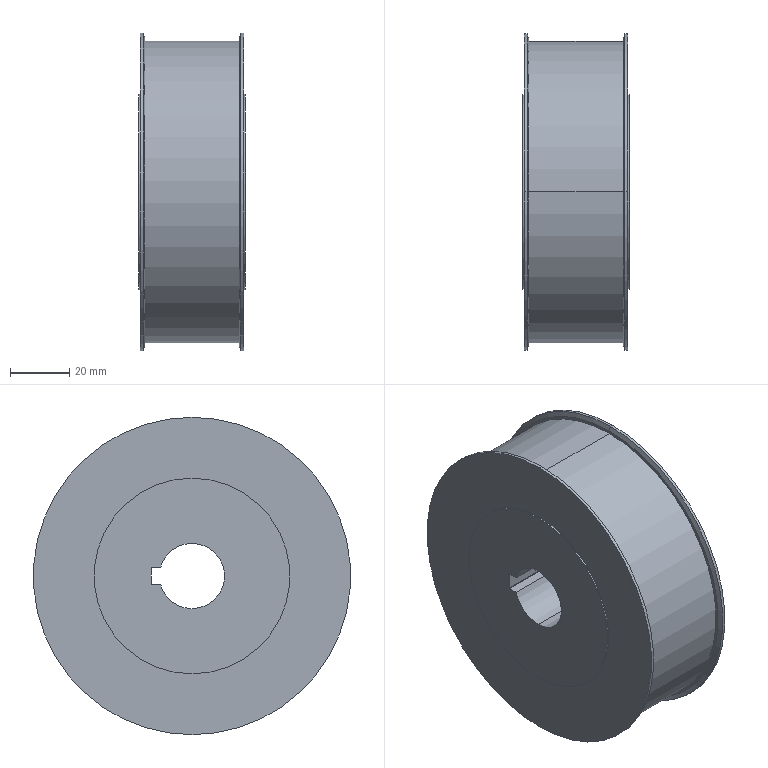Part | SolidWorks | features ICE 3, Fillet 1, Revolution 1 | 1 solid | 35 faces | box 36 x 107 x 107 mm | volume 274839 mm3 | cylinder 20 | plane 11 | cone 4 | commonest cylinder face diameters 66 x4 107 x4 22 x3 24.5 x3 0.4 x2 35 x2
STEP:
#1=CARTESIAN_POINT('',(11.,0.,12.25));
#2=VERTEX_POINT('',#1);
#3=CARTESIAN_POINT('',(11.,0.,-12.25));
#4=VERTEX_POINT('',#3);
#5=CARTESIAN_POINT('',(11.,0.,0.));
#6=DIRECTION('',(1.,0.,0.));
#7=DIRECTION('',(0.,0.,-1.));
#8=AXIS2_PLACEMENT_3D('',#5,#6,#7);
#9=CIRCLE('',#8,12.25);
#10=EDGE_CURVE('',#2,#4,#9,.T.);
#11=ORIENTED_EDGE('',*,*,#10,.F.);
#12=CARTESIAN_POINT('',(16.,0.,12.25));
#13=VERTEX_POINT('',#12);
#14=CARTESIAN_POINT('',(11.,0.,12.25));
#15=DIRECTION('',(1.,0.,0.));
#16=VECTOR('',#15,1000.);
#17=LINE('',#14,#16);
#18=EDGE_CURVE('',#2,#13,#17,.T.);
#19=ORIENTED_EDGE('',*,*,#18,.T.);
#20=CARTESIAN_POINT('',(16.,0.,-12.25));
#21=VERTEX_POINT('',#20);
#22=CARTESIAN_POINT('',(16.,0.,0.));
#23=DIRECTION('',(1.,0.,0.));
#24=DIRECTION('',(0.,0.,-1.));
#25=AXIS2_PLACEMENT_3D('',#22,#23,#24);
#26=CIRCLE('',#25,12.25);
#27=EDGE_CURVE('',#13,#21,#26,.T.);
#28=ORIENTED_EDGE('',*,*,#27,.T.);
#29=CARTESIAN_POINT('',(11.,0.,-12.25));
#30=DIRECTION('',(1.,0.,0.));
#31=VECTOR('',#30,1000.);
#32=LINE('',#29,#31);
#33=EDGE_CURVE('',#4,#21,#32,.T.);
#34=ORIENTED_EDGE('',*,*,#33,.F.);
#35=EDGE_LOOP('',(#11,#19,#28,#34));
#36=FACE_OUTER_BOUND('',#35,.T.);
#37=CARTESIAN_POINT('',(11.,0.,0.));
#38=DIRECTION('',(1.,0.,0.));
#39=DIRECTION('',(0.,0.,-1.));
#40=AXIS2_PLACEMENT_3D('',#37,#38,#39);
#41=CYLINDRICAL_SURFACE('',#40,12.25);
#42=ADVANCED_FACE('',(#36),#41,.F.);
#43=CARTESIAN_POINT('',(11.,11.877,-3.));
#44=VERTEX_POINT('',#43);
#45=CARTESIAN_POINT('',(11.,0.,0.));
#46=DIRECTION('',(1.,0.,0.));
#47=DIRECTION('',(0.,0.,-1.));
#48=AXIS2_PLACEMENT_3D('',#45,#46,#47);
#49=CIRCLE('',#48,12.25);
#50=EDGE_CURVE('',#4,#44,#49,.T.);
#51=ORIENTED_EDGE('',*,*,#50,.F.);
#52=ORIENTED_EDGE('',*,*,#33,.T.);
#53=CARTESIAN_POINT('',(16.,11.877,-3.));
#54=VERTEX_POINT('',#53);
#55=CARTESIAN_POINT('',(16.,0.,0.));
#56=DIRECTION('',(1.,0.,0.));
#57=DIRECTION('',(0.,0.,-1.));
#58=AXIS2_PLACEMENT_3D('',#55,#56,#57);
#59=CIRCLE('',#58,12.25);
#60=EDGE_CURVE('',#21,#54,#59,.T.);
#61=ORIENTED_EDGE('',*,*,#60,.T.);
#62=CARTESIAN_POINT('',(11.,11.877,-3.));
#63=DIRECTION('',(1.,0.,0.));
#64=VECTOR('',#63,1000.);
#65=LINE('',#62,#64);
#66=EDGE_CURVE('',#44,#54,#65,.T.);
#67=ORIENTED_EDGE('',*,*,#66,.F.);
#68=EDGE_LOOP('',(#51,#52,#61,#67));
#69=FACE_OUTER_BOUND('',#68,.T.);
#70=CARTESIAN_POINT('',(11.,0.,0.));
#71=DIRECTION('',(1.,0.,0.));
#72=DIRECTION('',(0.,0.,-1.));
#73=AXIS2_PLACEMENT_3D('',#70,#71,#72);
#74=CYLINDRICAL_SURFACE('',#73,12.25);
#75=ADVANCED_FACE('',(#69),#74,.F.);
#76=CARTESIAN_POINT('',(16.,0.,17.5));
#77=VERTEX_POINT('',#76);
#78=CARTESIAN_POINT('',(16.,0.,-17.5));
#79=VERTEX_POINT('',#78);
#80=CARTESIAN_POINT('',(16.,0.,0.));
#81=DIRECTION('',(1.,0.,0.));
#82=DIRECTION('',(0.,0.,-1.));
#83=AXIS2_PLACEMENT_3D('',#80,#81,#82);
#84=CIRCLE('',#83,17.5);
#85=EDGE_CURVE('',#77,#79,#84,.T.);
#86=ORIENTED_EDGE('',*,*,#85,.F.);
#87=CARTESIAN_POINT('',(18.,0.,17.5));
#88=VERTEX_POINT('',#87);
#89=CARTESIAN_POINT('',(16.,0.,17.5));
#90=DIRECTION('',(1.,0.,0.));
#91=VECTOR('',#90,1000.);
#92=LINE('',#89,#91);
#93=EDGE_CURVE('',#77,#88,#92,.T.);
#94=ORIENTED_EDGE('',*,*,#93,.T.);
#95=CARTESIAN_POINT('',(18.,0.,-17.5));
#96=VERTEX_POINT('',#95);
#97=CARTESIAN_POINT('',(18.,0.,0.));
#98=DIRECTION('',(1.,0.,0.));
#99=DIRECTION('',(0.,0.,-1.));
#100=AXIS2_PLACEMENT_3D('',#97,#98,#99);
#101=CIRCLE('',#100,17.5);
#102=EDGE_CURVE('',#88,#96,#101,.T.);
#103=ORIENTED_EDGE('',*,*,#102,.T.);
#104=CARTESIAN_POINT('',(16.,0.,-17.5));
#105=DIRECTION('',(1.,0.,0.));
#106=VECTOR('',#105,1000.);
#107=LINE('',#104,#106);
#108=EDGE_CURVE('',#79,#96,#107,.T.);
#109=ORIENTED_EDGE('',*,*,#108,.F.);
#110=EDGE_LOOP('',(#86,#94,#103,#109));
#111=FACE_OUTER_BOUND('',#110,.T.);
#112=CARTESIAN_POINT('',(16.,0.,0.));
#113=DIRECTION('',(1.,0.,0.));
#114=DIRECTION('',(0.,0.,-1.));
#115=AXIS2_PLACEMENT_3D('',#112,#113,#114);
#116=CYLINDRICAL_SURFACE('',#115,17.5);
#117=ADVANCED_FACE('',(#111),#116,.F.);
#118=CARTESIAN_POINT('',(-17.5,0.,33.));
#119=VERTEX_POINT('',#118);
#120=CARTESIAN_POINT('',(-17.5,0.,-33.));
#121=VERTEX_POINT('',#120);
#122=CARTESIAN_POINT('',(-17.5,0.,0.));
#123=DIRECTION('',(-1.,0.,0.));
#124=DIRECTION('',(0.,0.,1.));
#125=AXIS2_PLACEMENT_3D('',#122,#123,#124);
#126=CIRCLE('',#125,33.);
#127=EDGE_CURVE('',#119,#121,#126,.T.);
#128=ORIENTED_EDGE('',*,*,#127,.T.);
#129=CARTESIAN_POINT('',(-18.,0.,-33.));
#130=VERTEX_POINT('',#129);
#131=CARTESIAN_POINT('',(-18.,0.,-33.));
#132=DIRECTION('',(-1.,0.,0.));
#133=VECTOR('',#132,1000.);
#134=LINE('',#131,#133);
#135=EDGE_CURVE('',#121,#130,#134,.T.);
#136=ORIENTED_EDGE('',*,*,#135,.T.);
#137=CARTESIAN_POINT('',(-18.,0.,33.));
#138=VERTEX_POINT('',#137);
#139=CARTESIAN_POINT('',(-18.,0.,0.));
#140=DIRECTION('',(-1.,0.,0.));
#141=DIRECTION('',(0.,0.,1.));
#142=AXIS2_PLACEMENT_3D('',#139,#140,#141);
#143=CIRCLE('',#142,33.);
#144=EDGE_CURVE('',#138,#130,#143,.T.);
#145=ORIENTED_EDGE('',*,*,#144,.F.);
#146=CARTESIAN_POINT('',(-18.,0.,33.));
#147=DIRECTION('',(-1.,0.,0.));
#148=VECTOR('',#147,1000.);
#149=LINE('',#146,#148);
#150=EDGE_CURVE('',#119,#138,#149,.T.);
#151=ORIENTED_EDGE('',*,*,#150,.F.);
#152=EDGE_LOOP('',(#128,#136,#145,#151));
#153=FACE_OUTER_BOUND('',#152,.T.);
#154=CARTESIAN_POINT('',(-18.,0.,0.));
#155=DIRECTION('',(-1.,0.,0.));
#156=DIRECTION('',(0.,0.,1.));
#157=AXIS2_PLACEMENT_3D('',#154,#155,#156);
#158=CYLINDRICAL_SURFACE('',#157,33.);
#159=ADVANCED_FACE('',(#153),#158,.T.);
#160=CARTESIAN_POINT('',(-16.5,0.,53.5));
#161=VERTEX_POINT('',#160);
#162=CARTESIAN_POINT('',(-16.5,0.,-53.5));
#163=VERTEX_POINT('',#162);
#164=CARTESIAN_POINT('',(-16.5,0.,0.));
#165=DIRECTION('',(-1.,0.,0.));
#166=DIRECTION('',(0.,0.,1.));
#167=AXIS2_PLACEMENT_3D('',#164,#165,#166);
#168=CIRCLE('',#167,53.5);
#169=EDGE_CURVE('',#161,#163,#168,.T.);
#170=ORIENTED_EDGE('',*,*,#169,.T.);
#171=CARTESIAN_POINT('',(-17.5,0.,-53.5));
#172=VERTEX_POINT('',#171);
#173=CARTESIAN_POINT('',(-18.,0.,-53.5));
#174=DIRECTION('',(-1.,0.,0.));
#175=VECTOR('',#174,1000.);
#176=LINE('',#173,#175);
#177=EDGE_CURVE('',#163,#172,#176,.T.);
#178=ORIENTED_EDGE('',*,*,#177,.T.);
#179=CARTESIAN_POINT('',(-17.5,0.,53.5));
#180=VERTEX_POINT('',#179);
#181=CARTESIAN_POINT('',(-17.5,0.,0.));
#182=DIRECTION('',(-1.,0.,0.));
#183=DIRECTION('',(0.,0.,1.));
#184=AXIS2_PLACEMENT_3D('',#181,#182,#183);
#185=CIRCLE('',#184,53.5);
#186=EDGE_CURVE('',#180,#172,#185,.T.);
#187=ORIENTED_EDGE('',*,*,#186,.F.);
#188=CARTESIAN_POINT('',(-18.,0.,53.5));
#189=DIRECTION('',(-1.,0.,0.));
#190=VECTOR('',#189,1000.);
#191=LINE('',#188,#190);
#192=EDGE_CURVE('',#161,#180,#191,.T.);
#193=ORIENTED_EDGE('',*,*,#192,.F.);
#194=EDGE_LOOP('',(#170,#178,#187,#193));
#195=FACE_OUTER_BOUND('',#194,.T.);
#196=CARTESIAN_POINT('',(-18.,0.,0.));
#197=DIRECTION('',(-1.,0.,0.));
#198=DIRECTION('',(0.,0.,1.));
#199=AXIS2_PLACEMENT_3D('',#196,#197,#198);
#200=CYLINDRICAL_SURFACE('',#199,53.5);
#201=ADVANCED_FACE('',(#195),#200,.T.);
#202=CARTESIAN_POINT('',(-15.9,0.,51.9));
#203=VERTEX_POINT('',#202);
#204=CARTESIAN_POINT('',(-15.9,0.,-51.9));
#205=VERTEX_POINT('',#204);
#206=CARTESIAN_POINT('',(-15.9,0.,0.));
#207=DIRECTION('',(-1.,0.,0.));
#208=DIRECTION('',(0.,0.,1.));
#209=AXIS2_PLACEMENT_3D('',#206,#207,#208);
#210=CIRCLE('',#209,51.9);
#211=EDGE_CURVE('',#203,#205,#210,.T.);
#212=ORIENTED_EDGE('',*,*,#211,.T.);
#213=CARTESIAN_POINT('',(-15.9,0.,-51.9));
#214=DIRECTION('',(-0.3511,0.,-0.9363));
#215=VECTOR('',#214,1000.);
#216=LINE('',#213,#215);
#217=EDGE_CURVE('',#205,#163,#216,.T.);
#218=ORIENTED_EDGE('',*,*,#217,.T.);
#219=ORIENTED_EDGE('',*,*,#169,.F.);
#220=CARTESIAN_POINT('',(-15.9,0.,51.9));
#221=DIRECTION('',(-0.3511,0.,0.9363));
#222=VECTOR('',#221,1000.);
#223=LINE('',#220,#222);
#224=EDGE_CURVE('',#203,#161,#223,.T.);
#225=ORIENTED_EDGE('',*,*,#224,.F.);
#226=EDGE_LOOP('',(#212,#218,#219,#225));
#227=FACE_OUTER_BOUND('',#226,.T.);
#228=CARTESIAN_POINT('',(-15.9,0.,0.));
#229=DIRECTION('',(-1.,0.,0.));
#230=DIRECTION('',(0.,0.,1.));
#231=AXIS2_PLACEMENT_3D('',#228,#229,#230);
#232=CONICAL_SURFACE('',#231,51.9,1.212);
#233=ADVANCED_FACE('',(#227),#232,.T.);
#234=CARTESIAN_POINT('',(15.9,0.,50.9));
#235=VERTEX_POINT('',#234);
#236=CARTESIAN_POINT('',(15.9,0.,-50.9));
#237=VERTEX_POINT('',#236);
#238=CARTESIAN_POINT('',(15.9,0.,0.));
#239=DIRECTION('',(-1.,0.,0.));
#240=DIRECTION('',(0.,0.,1.));
#241=AXIS2_PLACEMENT_3D('',#238,#239,#240);
#242=CIRCLE('',#241,50.9);
#243=EDGE_CURVE('',#235,#237,#242,.T.);
#244=ORIENTED_EDGE('',*,*,#243,.T.);
#245=CARTESIAN_POINT('',(-15.9,0.,-50.9));
#246=VERTEX_POINT('',#245);
#247=CARTESIAN_POINT('',(-18.,0.,-50.9));
#248=DIRECTION('',(-1.,0.,0.));
#249=VECTOR('',#248,1000.);
#250=LINE('',#247,#249);
#251=EDGE_CURVE('',#237,#246,#250,.T.);
#252=ORIENTED_EDGE('',*,*,#251,.T.);
#253=CARTESIAN_POINT('',(-15.9,0.,50.9));
#254=VERTEX_POINT('',#253);
#255=CARTESIAN_POINT('',(-15.9,0.,0.));
#256=DIRECTION('',(-1.,0.,0.));
#257=DIRECTION('',(0.,0.,1.));
#258=AXIS2_PLACEMENT_3D('',#255,#256,#257);
#259=CIRCLE('',#258,50.9);
#260=EDGE_CURVE('',#254,#246,#259,.T.);
#261=ORIENTED_EDGE('',*,*,#260,.F.);
#262=CARTESIAN_POINT('',(-18.,0.,50.9));
#263=DIRECTION('',(-1.,0.,0.));
#264=VECTOR('',#263,1000.);
#265=LINE('',#262,#264);
#266=EDGE_CURVE('',#235,#254,#265,.T.);
#267=ORIENTED_EDGE('',*,*,#266,.F.);
#268=EDGE_LOOP('',(#244,#252,#261,#267));
#269=FACE_OUTER_BOUND('',#268,.T.);
#270=CARTESIAN_POINT('',(-18.,0.,0.));
#271=DIRECTION('',(-1.,0.,0.));
#272=DIRECTION('',(0.,0.,1.));
#273=AXIS2_PLACEMENT_3D('',#270,#271,#272);
#274=CYLINDRICAL_SURFACE('',#273,50.9);
#275=ADVANCED_FACE('',(#269),#274,.T.);
#276=CARTESIAN_POINT('',(15.9,0.,51.9));
#277=VERTEX_POINT('',#276);
#278=CARTESIAN_POINT('',(15.9,0.,-51.9));
#279=VERTEX_POINT('',#278);
#280=CARTESIAN_POINT('',(15.9,0.,0.));
#281=DIRECTION('',(-1.,0.,0.));
#282=DIRECTION('',(0.,0.,1.));
#283=AXIS2_PLACEMENT_3D('',#280,#281,#282);
#284=CIRCLE('',#283,51.9);
#285=EDGE_CURVE('',#277,#279,#284,.T.);
#286=ORIENTED_EDGE('',*,*,#285,.F.);
#287=CARTESIAN_POINT('',(16.5,0.,53.5));
#288=VERTEX_POINT('',#287);
#289=CARTESIAN_POINT('',(16.5,0.,53.5));
#290=DIRECTION('',(0.3511,0.,0.9363));
#291=VECTOR('',#290,1000.);
#292=LINE('',#289,#291);
#293=EDGE_CURVE('',#277,#288,#292,.T.);
#294=ORIENTED_EDGE('',*,*,#293,.T.);
#295=CARTESIAN_POINT('',(16.5,0.,-53.5));
#296=VERTEX_POINT('',#295);
#297=CARTESIAN_POINT('',(16.5,0.,0.));
#298=DIRECTION('',(-1.,0.,0.));
#299=DIRECTION('',(0.,0.,1.));
#300=AXIS2_PLACEMENT_3D('',#297,#298,#299);
#301=CIRCLE('',#300,53.5);
#302=EDGE_CURVE('',#288,#296,#301,.T.);
#303=ORIENTED_EDGE('',*,*,#302,.T.);
#304=CARTESIAN_POINT('',(16.5,0.,-53.5));
#305=DIRECTION('',(0.3511,0.,-0.9363));
#306=VECTOR('',#305,1000.);
#307=LINE('',#304,#306);
#308=EDGE_CURVE('',#279,#296,#307,.T.);
#309=ORIENTED_EDGE('',*,*,#308,.F.);
#310=EDGE_LOOP('',(#286,#294,#303,#309));
#311=FACE_OUTER_BOUND('',#310,.T.);
#312=CARTESIAN_POINT('',(16.5,0.,0.));
#313=DIRECTION('',(1.,0.,0.));
#314=DIRECTION('',(0.,0.,-1.));
#315=AXIS2_PLACEMENT_3D('',#312,#313,#314);
#316=CONICAL_SURFACE('',#315,53.5,1.212);
#317=ADVANCED_FACE('',(#311),#316,.T.);
#318=CARTESIAN_POINT('',(17.5,0.,53.5));
#319=VERTEX_POINT('',#318);
#320=CARTESIAN_POINT('',(17.5,0.,-53.5));
#321=VERTEX_POINT('',#320);
#322=CARTESIAN_POINT('',(17.5,0.,0.));
#323=DIRECTION('',(-1.,0.,0.));
#324=DIRECTION('',(0.,0.,1.));
#325=AXIS2_PLACEMENT_3D('',#322,#323,#324);
#326=CIRCLE('',#325,53.5);
#327=EDGE_CURVE('',#319,#321,#326,.T.);
#328=ORIENTED_EDGE('',*,*,#327,.T.);
#329=CARTESIAN_POINT('',(-18.,0.,-53.5));
#330=DIRECTION('',(-1.,0.,0.));
#331=VECTOR('',#330,1000.);
#332=LINE('',#329,#331);
#333=EDGE_CURVE('',#321,#296,#332,.T.);
#334=ORIENTED_EDGE('',*,*,#333,.T.);
#335=ORIENTED_EDGE('',*,*,#302,.F.);
#336=CARTESIAN_POINT('',(-18.,0.,53.5));
#337=DIRECTION('',(-1.,0.,0.));
#338=VECTOR('',#337,1000.);
#339=LINE('',#336,#338);
#340=EDGE_CURVE('',#319,#288,#339,.T.);
#341=ORIENTED_EDGE('',*,*,#340,.F.);
#342=EDGE_LOOP('',(#328,#334,#335,#341));
#343=FACE_OUTER_BOUND('',#342,.T.);
#344=CARTESIAN_POINT('',(-18.,0.,0.));
#345=DIRECTION('',(-1.,0.,0.));
#346=DIRECTION('',(0.,0.,1.));
#347=AXIS2_PLACEMENT_3D('',#344,#345,#346);
#348=CYLINDRICAL_SURFACE('',#347,53.5);
#349=ADVANCED_FACE('',(#343),#348,.T.);
#350=CARTESIAN_POINT('',(18.,0.,33.));
#351=VERTEX_POINT('',#350);
#352=CARTESIAN_POINT('',(18.,0.,-33.));
#353=VERTEX_POINT('',#352);
#354=CARTESIAN_POINT('',(18.,0.,0.));
#355=DIRECTION('',(-1.,0.,0.));
#356=DIRECTION('',(0.,0.,1.));
#357=AXIS2_PLACEMENT_3D('',#354,#355,#356);
#358=CIRCLE('',#357,33.);
#359=EDGE_CURVE('',#351,#353,#358,.T.);
#360=ORIENTED_EDGE('',*,*,#359,.T.);
#361=CARTESIAN_POINT('',(17.5,0.,-33.));
#362=VERTEX_POINT('',#361);
#363=CARTESIAN_POINT('',(-18.,0.,-33.));
#364=DIRECTION('',(-1.,0.,0.));
#365=VECTOR('',#364,1000.);
#366=LINE('',#363,#365);
#367=EDGE_CURVE('',#353,#362,#366,.T.);
#368=ORIENTED_EDGE('',*,*,#367,.T.);
#369=CARTESIAN_POINT('',(17.5,0.,33.));
#370=VERTEX_POINT('',#369);
#371=CARTESIAN_POINT('',(17.5,0.,0.));
#372=DIRECTION('',(-1.,0.,0.));
#373=DIRECTION('',(0.,0.,1.));
#374=AXIS2_PLACEMENT_3D('',#371,#372,#373);
#375=CIRCLE('',#374,33.);
#376=EDGE_CURVE('',#370,#362,#375,.T.);
#377=ORIENTED_EDGE('',*,*,#376,.F.);
#378=CARTESIAN_POINT('',(-18.,0.,33.));
#379=DIRECTION('',(-1.,0.,0.));
#380=VECTOR('',#379,1000.);
#381=LINE('',#378,#380);
#382=EDGE_CURVE('',#351,#370,#381,.T.);
#383=ORIENTED_EDGE('',*,*,#382,.F.);
#384=EDGE_LOOP('',(#360,#368,#377,#383));
#385=FACE_OUTER_BOUND('',#384,.T.);
#386=CARTESIAN_POINT('',(-18.,0.,0.));
#387=DIRECTION('',(-1.,0.,0.));
#388=DIRECTION('',(0.,0.,1.));
#389=AXIS2_PLACEMENT_3D('',#386,#387,#388);
#390=CYLINDRICAL_SURFACE('',#389,33.);
#391=ADVANCED_FACE('',(#385),#390,.T.);
#392=CARTESIAN_POINT('',(-18.,0.,11.));
#393=VERTEX_POINT('',#392);
#394=CARTESIAN_POINT('',(-18.,0.,-11.));
#395=VERTEX_POINT('',#394);
#396=CARTESIAN_POINT('',(-18.,0.,0.));
#397=DIRECTION('',(1.,0.,0.));
#398=DIRECTION('',(0.,0.,-1.));
#399=AXIS2_PLACEMENT_3D('',#396,#397,#398);
#400=CIRCLE('',#399,11.);
#401=EDGE_CURVE('',#393,#395,#400,.T.);
#402=ORIENTED_EDGE('',*,*,#401,.F.);
#403=CARTESIAN_POINT('',(11.,0.,11.));
#404=VERTEX_POINT('',#403);
#405=CARTESIAN_POINT('',(-18.,0.,11.));
#406=DIRECTION('',(1.,0.,0.));
#407=VECTOR('',#406,1000.);
#408=LINE('',#405,#407);
#409=EDGE_CURVE('',#393,#404,#408,.T.);
#410=ORIENTED_EDGE('',*,*,#409,.T.);
#411=CARTESIAN_POINT('',(11.,0.,-11.));
#412=VERTEX_POINT('',#411);
#413=CARTESIAN_POINT('',(11.,0.,0.));
#414=DIRECTION('',(-1.,0.,0.));
#415=DIRECTION('',(0.,0.,-1.));
#416=AXIS2_PLACEMENT_3D('',#413,#414,#415);
#417=CIRCLE('',#416,11.);
#418=EDGE_CURVE('',#412,#404,#417,.T.);
#419=ORIENTED_EDGE('',*,*,#418,.F.);
#420=CARTESIAN_POINT('',(-18.,0.,-11.));
#421=DIRECTION('',(1.,0.,0.));
#422=VECTOR('',#421,1000.);
#423=LINE('',#420,#422);
#424=EDGE_CURVE('',#395,#412,#423,.T.);
#425=ORIENTED_EDGE('',*,*,#424,.F.);
#426=EDGE_LOOP('',(#402,#410,#419,#425));
#427=FACE_OUTER_BOUND('',#426,.T.);
#428=CARTESIAN_POINT('',(-18.,0.,0.));
#429=DIRECTION('',(1.,0.,0.));
#430=DIRECTION('',(0.,0.,-1.));
#431=AXIS2_PLACEMENT_3D('',#428,#429,#430);
#432=CYLINDRICAL_SURFACE('',#431,11.);
#433=ADVANCED_FACE('',(#427),#432,.F.);
#434=CARTESIAN_POINT('',(-18.,10.583,-3.));
#435=VERTEX_POINT('',#434);
#436=CARTESIAN_POINT('',(-18.,0.,0.));
#437=DIRECTION('',(1.,0.,0.));
#438=DIRECTION('',(0.,0.,-1.));
#439=AXIS2_PLACEMENT_3D('',#436,#437,#438);
#440=CIRCLE('',#439,11.);
#441=EDGE_CURVE('',#395,#435,#440,.T.);
#442=ORIENTED_EDGE('',*,*,#441,.F.);
#443=ORIENTED_EDGE('',*,*,#424,.T.);
#444=CARTESIAN_POINT('',(11.,10.583,-3.));
#445=VERTEX_POINT('',#444);
#446=CARTESIAN_POINT('',(11.,0.,0.));
#447=DIRECTION('',(-1.,0.,0.));
#448=DIRECTION('',(0.,0.,-1.));
#449=AXIS2_PLACEMENT_3D('',#446,#447,#448);
#450=CIRCLE('',#449,11.);
#451=EDGE_CURVE('',#445,#412,#450,.T.);
#452=ORIENTED_EDGE('',*,*,#451,.F.);
#453=CARTESIAN_POINT('',(-18.,10.583,-3.));
#454=DIRECTION('',(1.,0.,0.));
#455=VECTOR('',#454,1000.);
#456=LINE('',#453,#455);
#457=EDGE_CURVE('',#435,#445,#456,.T.);
#458=ORIENTED_EDGE('',*,*,#457,.F.);
#459=EDGE_LOOP('',(#442,#443,#452,#458));
#460=FACE_OUTER_BOUND('',#459,.T.);
#461=CARTESIAN_POINT('',(-18.,0.,0.));
#462=DIRECTION('',(1.,0.,0.));
#463=DIRECTION('',(0.,0.,-1.));
#464=AXIS2_PLACEMENT_3D('',#461,#462,#463);
#465=CYLINDRICAL_SURFACE('',#464,11.);
#466=ADVANCED_FACE('',(#460),#465,.F.);
#467=ORIENTED_EDGE('',*,*,#409,.F.);
#468=CARTESIAN_POINT('',(-18.,10.583,3.));
#469=VERTEX_POINT('',#468);
#470=CARTESIAN_POINT('',(-18.,0.,0.));
#471=DIRECTION('',(1.,0.,0.));
#472=DIRECTION('',(0.,0.,-1.));
#473=AXIS2_PLACEMENT_3D('',#470,#471,#472);
#474=CIRCLE('',#473,11.);
#475=EDGE_CURVE('',#469,#393,#474,.T.);
#476=ORIENTED_EDGE('',*,*,#475,.F.);
#477=CARTESIAN_POINT('',(11.,10.583,3.));
#478=VERTEX_POINT('',#477);
#479=CARTESIAN_POINT('',(-18.,10.583,3.));
#480=DIRECTION('',(1.,0.,0.));
#481=VECTOR('',#480,1000.);
#482=LINE('',#479,#481);
#483=EDGE_CURVE('',#469,#478,#482,.T.);
#484=ORIENTED_EDGE('',*,*,#483,.T.);
#485=CARTESIAN_POINT('',(11.,0.,0.));
#486=DIRECTION('',(-1.,0.,0.));
#487=DIRECTION('',(0.,0.,-1.));
#488=AXIS2_PLACEMENT_3D('',#485,#486,#487);
#489=CIRCLE('',#488,11.);
#490=EDGE_CURVE('',#404,#478,#489,.T.);
#491=ORIENTED_EDGE('',*,*,#490,.F.);
#492=EDGE_LOOP('',(#467,#476,#484,#491));
#493=FACE_OUTER_BOUND('',#492,.T.);
#494=CARTESIAN_POINT('',(-18.,0.,0.));
#495=DIRECTION('',(1.,0.,0.));
#496=DIRECTION('',(0.,0.,-1.));
#497=AXIS2_PLACEMENT_3D('',#494,#495,#496);
#498=CYLINDRICAL_SURFACE('',#497,11.);
#499=ADVANCED_FACE('',(#493),#498,.F.);
#500=CARTESIAN_POINT('',(18.,0.,0.));
#501=DIRECTION('',(1.,0.,0.));
#502=DIRECTION('',(0.,0.,-1.));
#503=AXIS2_PLACEMENT_3D('',#500,#501,#502);
#504=CIRCLE('',#503,17.5);
#505=EDGE_CURVE('',#96,#88,#504,.T.);
#506=ORIENTED_EDGE('',*,*,#505,.F.);
#507=ORIENTED_EDGE('',*,*,#102,.F.);
#508=EDGE_LOOP('',(#506,#507));
#509=FACE_BOUND('',#508,.T.);
#510=ORIENTED_EDGE('',*,*,#359,.F.);
#511=CARTESIAN_POINT('',(18.,0.,0.));
#512=DIRECTION('',(-1.,0.,0.));
#513=DIRECTION('',(0.,0.,1.));
#514=AXIS2_PLACEMENT_3D('',#511,#512,#513);
#515=CIRCLE('',#514,33.);
#516=EDGE_CURVE('',#353,#351,#515,.T.);
#517=ORIENTED_EDGE('',*,*,#516,.F.);
#518=EDGE_LOOP('',(#510,#517));
#519=FACE_OUTER_BOUND('',#518,.T.);
#520=CARTESIAN_POINT('',(18.,0.,0.));
#521=DIRECTION('',(-1.,0.,0.));
#522=DIRECTION('',(0.,0.,1.));
#523=AXIS2_PLACEMENT_3D('',#520,#521,#522);
#524=PLANE('',#523);
#525=ADVANCED_FACE('',(#509,#519),#524,.F.);
#526=ORIENTED_EDGE('',*,*,#367,.F.);
#527=ORIENTED_EDGE('',*,*,#516,.T.);
#528=ORIENTED_EDGE('',*,*,#382,.T.);
#529=CARTESIAN_POINT('',(17.5,0.,0.));
#530=DIRECTION('',(-1.,0.,0.));
#531=DIRECTION('',(0.,0.,1.));
#532=AXIS2_PLACEMENT_3D('',#529,#530,#531);
#533=CIRCLE('',#532,33.);
#534=EDGE_CURVE('',#362,#370,#533,.T.);
#535=ORIENTED_EDGE('',*,*,#534,.F.);
#536=EDGE_LOOP('',(#526,#527,#528,#535));
#537=FACE_OUTER_BOUND('',#536,.T.);
#538=CARTESIAN_POINT('',(-18.,0.,0.));
#539=DIRECTION('',(-1.,0.,0.));
#540=DIRECTION('',(0.,0.,1.));
#541=AXIS2_PLACEMENT_3D('',#538,#539,#540);
#542=CYLINDRICAL_SURFACE('',#541,33.);
#543=ADVANCED_FACE('',(#537),#542,.T.);
#544=ORIENTED_EDGE('',*,*,#327,.F.);
#545=CARTESIAN_POINT('',(17.5,0.,0.));
#546=DIRECTION('',(-1.,0.,0.));
#547=DIRECTION('',(0.,0.,1.));
#548=AXIS2_PLACEMENT_3D('',#545,#546,#547);
#549=CIRCLE('',#548,53.5);
#550=EDGE_CURVE('',#321,#319,#549,.T.);
#551=ORIENTED_EDGE('',*,*,#550,.F.);
#552=EDGE_LOOP('',(#544,#551));
#553=FACE_OUTER_BOUND('',#552,.T.);
#554=ORIENTED_EDGE('',*,*,#376,.T.);
#555=ORIENTED_EDGE('',*,*,#534,.T.);
#556=EDGE_LOOP('',(#554,#555));
#557=FACE_BOUND('',#556,.T.);
#558=CARTESIAN_POINT('',(17.5,33.,0.));
#559=DIRECTION('',(-1.,0.,0.));
#560=DIRECTION('',(0.,0.,1.));
#561=AXIS2_PLACEMENT_3D('',#558,#559,#560);
#562=PLANE('',#561);
#563=ADVANCED_FACE('',(#553,#557),#562,.F.);
#564=ORIENTED_EDGE('',*,*,#333,.F.);
#565=ORIENTED_EDGE('',*,*,#550,.T.);
#566=ORIENTED_EDGE('',*,*,#340,.T.);
#567=CARTESIAN_POINT('',(16.5,0.,0.));
#568=DIRECTION('',(-1.,0.,0.));
#569=DIRECTION('',(0.,0.,1.));
#570=AXIS2_PLACEMENT_3D('',#567,#568,#569);
#571=CIRCLE('',#570,53.5);
#572=EDGE_CURVE('',#296,#288,#571,.T.);
#573=ORIENTED_EDGE('',*,*,#572,.F.);
#574=EDGE_LOOP('',(#564,#565,#566,#573));
#575=FACE_OUTER_BOUND('',#574,.T.);
#576=CARTESIAN_POINT('',(-18.,0.,0.));
#577=DIRECTION('',(-1.,0.,0.));
#578=DIRECTION('',(0.,0.,1.));
#579=AXIS2_PLACEMENT_3D('',#576,#577,#578);
#580=CYLINDRICAL_SURFACE('',#579,53.5);
#581=ADVANCED_FACE('',(#575),#580,.T.);
#582=ORIENTED_EDGE('',*,*,#293,.F.);
#583=CARTESIAN_POINT('',(15.9,0.,0.));
#584=DIRECTION('',(-1.,0.,0.));
#585=DIRECTION('',(0.,0.,1.));
#586=AXIS2_PLACEMENT_3D('',#583,#584,#585);
#587=CIRCLE('',#586,51.9);
#588=EDGE_CURVE('',#279,#277,#587,.T.);
#589=ORIENTED_EDGE('',*,*,#588,.F.);
#590=ORIENTED_EDGE('',*,*,#308,.T.);
#591=ORIENTED_EDGE('',*,*,#572,.T.);
#592=EDGE_LOOP('',(#582,#589,#590,#591));
#593=FACE_OUTER_BOUND('',#592,.T.);
#594=CARTESIAN_POINT('',(16.5,0.,0.));
#595=DIRECTION('',(1.,0.,0.));
#596=DIRECTION('',(0.,0.,-1.));
#597=AXIS2_PLACEMENT_3D('',#594,#595,#596);
#598=CONICAL_SURFACE('',#597,53.5,1.212);
#599=ADVANCED_FACE('',(#593),#598,.T.);
#600=ORIENTED_EDGE('',*,*,#243,.F.);
#601=CARTESIAN_POINT('',(15.9,0.,0.));
#602=DIRECTION('',(-1.,0.,0.));
#603=DIRECTION('',(0.,0.,1.));
#604=AXIS2_PLACEMENT_3D('',#601,#602,#603);
#605=CIRCLE('',#604,50.9);
#606=EDGE_CURVE('',#237,#235,#605,.T.);
#607=ORIENTED_EDGE('',*,*,#606,.F.);
#608=EDGE_LOOP('',(#600,#607));
#609=FACE_BOUND('',#608,.T.);
#610=ORIENTED_EDGE('',*,*,#588,.T.);
#611=ORIENTED_EDGE('',*,*,#285,.T.);
#612=EDGE_LOOP('',(#610,#611));
#613=FACE_OUTER_BOUND('',#612,.T.);
#614=CARTESIAN_POINT('',(15.9,51.9,0.));
#615=DIRECTION('',(1.,0.,0.));
#616=DIRECTION('',(0.,0.,-1.));
#617=AXIS2_PLACEMENT_3D('',#614,#615,#616);
#618=PLANE('',#617);
#619=ADVANCED_FACE('',(#609,#613),#618,.F.);
#620=ORIENTED_EDGE('',*,*,#251,.F.);
#621=ORIENTED_EDGE('',*,*,#606,.T.);
#622=ORIENTED_EDGE('',*,*,#266,.T.);
#623=CARTESIAN_POINT('',(-15.9,0.,0.));
#624=DIRECTION('',(-1.,0.,0.));
#625=DIRECTION('',(0.,0.,1.));
#626=AXIS2_PLACEMENT_3D('',#623,#624,#625);
#627=CIRCLE('',#626,50.9);
#628=EDGE_CURVE('',#246,#254,#627,.T.);
#629=ORIENTED_EDGE('',*,*,#628,.F.);
#630=EDGE_LOOP('',(#620,#621,#622,#629));
#631=FACE_OUTER_BOUND('',#630,.T.);
#632=CARTESIAN_POINT('',(-18.,0.,0.));
#633=DIRECTION('',(-1.,0.,0.));
#634=DIRECTION('',(0.,0.,1.));
#635=AXIS2_PLACEMENT_3D('',#632,#633,#634);
#636=CYLINDRICAL_SURFACE('',#635,50.9);
#637=ADVANCED_FACE('',(#631),#636,.T.);
#638=ORIENTED_EDGE('',*,*,#211,.F.);
#639=CARTESIAN_POINT('',(-15.9,0.,0.));
#640=DIRECTION('',(-1.,0.,0.));
#641=DIRECTION('',(0.,0.,1.));
#642=AXIS2_PLACEMENT_3D('',#639,#640,#641);
#643=CIRCLE('',#642,51.9);
#644=EDGE_CURVE('',#205,#203,#643,.T.);
#645=ORIENTED_EDGE('',*,*,#644,.F.);
#646=EDGE_LOOP('',(#638,#645));
#647=FACE_OUTER_BOUND('',#646,.T.);
#648=ORIENTED_EDGE('',*,*,#260,.T.);
#649=ORIENTED_EDGE('',*,*,#628,.T.);
#650=EDGE_LOOP('',(#648,#649));
#651=FACE_BOUND('',#650,.T.);
#652=CARTESIAN_POINT('',(-15.9,51.9,0.));
#653=DIRECTION('',(-1.,0.,0.));
#654=DIRECTION('',(0.,0.,1.));
#655=AXIS2_PLACEMENT_3D('',#652,#653,#654);
#656=PLANE('',#655);
#657=ADVANCED_FACE('',(#647,#651),#656,.F.);
#658=ORIENTED_EDGE('',*,*,#217,.F.);
#659=ORIENTED_EDGE('',*,*,#644,.T.);
#660=ORIENTED_EDGE('',*,*,#224,.T.);
#661=CARTESIAN_POINT('',(-16.5,0.,0.));
#662=DIRECTION('',(-1.,0.,0.));
#663=DIRECTION('',(0.,0.,1.));
#664=AXIS2_PLACEMENT_3D('',#661,#662,#663);
#665=CIRCLE('',#664,53.5);
#666=EDGE_CURVE('',#163,#161,#665,.T.);
#667=ORIENTED_EDGE('',*,*,#666,.F.);
#668=EDGE_LOOP('',(#658,#659,#660,#667));
#669=FACE_OUTER_BOUND('',#668,.T.);
#670=CARTESIAN_POINT('',(-15.9,0.,0.));
#671=DIRECTION('',(-1.,0.,0.));
#672=DIRECTION('',(0.,0.,1.));
#673=AXIS2_PLACEMENT_3D('',#670,#671,#672);
#674=CONICAL_SURFACE('',#673,51.9,1.212);
#675=ADVANCED_FACE('',(#669),#674,.T.);
#676=ORIENTED_EDGE('',*,*,#177,.F.);
#677=ORIENTED_EDGE('',*,*,#666,.T.);
#678=ORIENTED_EDGE('',*,*,#192,.T.);
#679=CARTESIAN_POINT('',(-17.5,0.,0.));
#680=DIRECTION('',(-1.,0.,0.));
#681=DIRECTION('',(0.,0.,1.));
#682=AXIS2_PLACEMENT_3D('',#679,#680,#681);
#683=CIRCLE('',#682,53.5);
#684=EDGE_CURVE('',#172,#180,#683,.T.);
#685=ORIENTED_EDGE('',*,*,#684,.F.);
#686=EDGE_LOOP('',(#676,#677,#678,#685));
#687=FACE_OUTER_BOUND('',#686,.T.);
#688=CARTESIAN_POINT('',(-18.,0.,0.));
#689=DIRECTION('',(-1.,0.,0.));
#690=DIRECTION('',(0.,0.,1.));
#691=AXIS2_PLACEMENT_3D('',#688,#689,#690);
#692=CYLINDRICAL_SURFACE('',#691,53.5);
#693=ADVANCED_FACE('',(#687),#692,.T.);
#694=ORIENTED_EDGE('',*,*,#127,.F.);
#695=CARTESIAN_POINT('',(-17.5,0.,0.));
#696=DIRECTION('',(-1.,0.,0.));
#697=DIRECTION('',(0.,0.,1.));
#698=AXIS2_PLACEMENT_3D('',#695,#696,#697);
#699=CIRCLE('',#698,33.);
#700=EDGE_CURVE('',#121,#119,#699,.T.);
#701=ORIENTED_EDGE('',*,*,#700,.F.);
#702=EDGE_LOOP('',(#694,#701));
#703=FACE_BOUND('',#702,.T.);
#704=ORIENTED_EDGE('',*,*,#186,.T.);
#705=ORIENTED_EDGE('',*,*,#684,.T.);
#706=EDGE_LOOP('',(#704,#705));
#707=FACE_OUTER_BOUND('',#706,.T.);
#708=CARTESIAN_POINT('',(-17.5,33.,0.));
#709=DIRECTION('',(1.,0.,0.));
#710=DIRECTION('',(0.,0.,-1.));
#711=AXIS2_PLACEMENT_3D('',#708,#709,#710);
#712=PLANE('',#711);
#713=ADVANCED_FACE('',(#703,#707),#712,.F.);
#714=ORIENTED_EDGE('',*,*,#135,.F.);
#715=ORIENTED_EDGE('',*,*,#700,.T.);
#716=ORIENTED_EDGE('',*,*,#150,.T.);
#717=CARTESIAN_POINT('',(-18.,0.,0.));
#718=DIRECTION('',(-1.,0.,0.));
#719=DIRECTION('',(0.,0.,1.));
#720=AXIS2_PLACEMENT_3D('',#717,#718,#719);
#721=CIRCLE('',#720,33.);
#722=EDGE_CURVE('',#130,#138,#721,.T.);
#723=ORIENTED_EDGE('',*,*,#722,.F.);
#724=EDGE_LOOP('',(#714,#715,#716,#723));
#725=FACE_OUTER_BOUND('',#724,.T.);
#726=CARTESIAN_POINT('',(-18.,0.,0.));
#727=DIRECTION('',(-1.,0.,0.));
#728=DIRECTION('',(0.,0.,1.));
#729=AXIS2_PLACEMENT_3D('',#726,#727,#728);
#730=CYLINDRICAL_SURFACE('',#729,33.);
#731=ADVANCED_FACE('',(#725),#730,.T.);
#732=CARTESIAN_POINT('',(-18.,13.6,-3.));
#733=VERTEX_POINT('',#732);
#734=CARTESIAN_POINT('',(-18.,10.583,-3.));
#735=DIRECTION('',(0.,1.,0.));
#736=VECTOR('',#735,1000.);
#737=LINE('',#734,#736);
#738=EDGE_CURVE('',#435,#733,#737,.T.);
#739=ORIENTED_EDGE('',*,*,#738,.T.);
#740=CARTESIAN_POINT('',(-18.,13.8,-2.8));
#741=VERTEX_POINT('',#740);
#742=CARTESIAN_POINT('',(-18.,13.6,-2.8));
#743=DIRECTION('',(1.,0.,0.));
#744=DIRECTION('',(0.,0.,-1.));
#745=AXIS2_PLACEMENT_3D('',#742,#743,#744);
#746=CIRCLE('',#745,0.2);
#747=EDGE_CURVE('',#733,#741,#746,.T.);
#748=ORIENTED_EDGE('',*,*,#747,.T.);
#749=CARTESIAN_POINT('',(-18.,13.8,2.8));
#750=VERTEX_POINT('',#749);
#751=CARTESIAN_POINT('',(-18.,13.8,3.));
#752=DIRECTION('',(0.,0.,1.));
#753=VECTOR('',#752,1000.);
#754=LINE('',#751,#753);
#755=EDGE_CURVE('',#741,#750,#754,.T.);
#756=ORIENTED_EDGE('',*,*,#755,.T.);
#757=CARTESIAN_POINT('',(-18.,13.6,3.));
#758=VERTEX_POINT('',#757);
#759=CARTESIAN_POINT('',(-18.,13.6,2.8));
#760=DIRECTION('',(1.,0.,0.));
#761=DIRECTION('',(0.,0.,-1.));
#762=AXIS2_PLACEMENT_3D('',#759,#760,#761);
#763=CIRCLE('',#762,0.2);
#764=EDGE_CURVE('',#750,#758,#763,.T.);
#765=ORIENTED_EDGE('',*,*,#764,.T.);
#766=CARTESIAN_POINT('',(-18.,10.583,3.));
#767=DIRECTION('',(0.,-1.,0.));
#768=VECTOR('',#767,1000.);
#769=LINE('',#766,#768);
#770=EDGE_CURVE('',#758,#469,#769,.T.);
#771=ORIENTED_EDGE('',*,*,#770,.T.);
#772=ORIENTED_EDGE('',*,*,#475,.T.);
#773=ORIENTED_EDGE('',*,*,#401,.T.);
#774=ORIENTED_EDGE('',*,*,#441,.T.);
#775=EDGE_LOOP('',(#739,#748,#756,#765,#771,#772,#773,#774));
#776=FACE_BOUND('',#775,.T.);
#777=ORIENTED_EDGE('',*,*,#144,.T.);
#778=ORIENTED_EDGE('',*,*,#722,.T.);
#779=EDGE_LOOP('',(#777,#778));
#780=FACE_OUTER_BOUND('',#779,.T.);
#781=CARTESIAN_POINT('',(-18.,0.,0.));
#782=DIRECTION('',(1.,0.,0.));
#783=DIRECTION('',(0.,0.,-1.));
#784=AXIS2_PLACEMENT_3D('',#781,#782,#783);
#785=PLANE('',#784);
#786=ADVANCED_FACE('',(#776,#780),#785,.F.);
#787=ORIENTED_EDGE('',*,*,#93,.F.);
#788=CARTESIAN_POINT('',(16.,0.,0.));
#789=DIRECTION('',(1.,0.,0.));
#790=DIRECTION('',(0.,0.,-1.));
#791=AXIS2_PLACEMENT_3D('',#788,#789,#790);
#792=CIRCLE('',#791,17.5);
#793=EDGE_CURVE('',#79,#77,#792,.T.);
#794=ORIENTED_EDGE('',*,*,#793,.F.);
#795=ORIENTED_EDGE('',*,*,#108,.T.);
#796=ORIENTED_EDGE('',*,*,#505,.T.);
#797=EDGE_LOOP('',(#787,#794,#795,#796));
#798=FACE_OUTER_BOUND('',#797,.T.);
#799=CARTESIAN_POINT('',(16.,0.,0.));
#800=DIRECTION('',(1.,0.,0.));
#801=DIRECTION('',(0.,0.,-1.));
#802=AXIS2_PLACEMENT_3D('',#799,#800,#801);
#803=CYLINDRICAL_SURFACE('',#802,17.5);
#804=ADVANCED_FACE('',(#798),#803,.F.);
#805=CARTESIAN_POINT('',(16.,11.877,3.));
#806=VERTEX_POINT('',#805);
#807=CARTESIAN_POINT('',(16.,0.,0.));
#808=DIRECTION('',(1.,0.,0.));
#809=DIRECTION('',(0.,0.,-1.));
#810=AXIS2_PLACEMENT_3D('',#807,#808,#809);
#811=CIRCLE('',#810,12.25);
#812=EDGE_CURVE('',#806,#13,#811,.T.);
#813=ORIENTED_EDGE('',*,*,#812,.F.);
#814=CARTESIAN_POINT('',(16.,13.6,3.));
#815=VERTEX_POINT('',#814);
#816=CARTESIAN_POINT('',(16.,10.583,3.));
#817=DIRECTION('',(0.,-1.,0.));
#818=VECTOR('',#817,1000.);
#819=LINE('',#816,#818);
#820=EDGE_CURVE('',#815,#806,#819,.T.);
#821=ORIENTED_EDGE('',*,*,#820,.F.);
#822=CARTESIAN_POINT('',(16.,13.8,2.8));
#823=VERTEX_POINT('',#822);
#824=CARTESIAN_POINT('',(16.,13.6,2.8));
#825=DIRECTION('',(-1.,0.,0.));
#826=DIRECTION('',(0.,0.,-1.));
#827=AXIS2_PLACEMENT_3D('',#824,#825,#826);
#828=CIRCLE('',#827,0.2);
#829=EDGE_CURVE('',#815,#823,#828,.T.);
#830=ORIENTED_EDGE('',*,*,#829,.T.);
#831=CARTESIAN_POINT('',(16.,13.8,-2.8));
#832=VERTEX_POINT('',#831);
#833=CARTESIAN_POINT('',(16.,13.8,3.));
#834=DIRECTION('',(0.,0.,1.));
#835=VECTOR('',#834,1000.);
#836=LINE('',#833,#835);
#837=EDGE_CURVE('',#832,#823,#836,.T.);
#838=ORIENTED_EDGE('',*,*,#837,.F.);
#839=CARTESIAN_POINT('',(16.,13.6,-3.));
#840=VERTEX_POINT('',#839);
#841=CARTESIAN_POINT('',(16.,13.6,-2.8));
#842=DIRECTION('',(-1.,0.,0.));
#843=DIRECTION('',(0.,0.,-1.));
#844=AXIS2_PLACEMENT_3D('',#841,#842,#843);
#845=CIRCLE('',#844,0.2);
#846=EDGE_CURVE('',#832,#840,#845,.T.);
#847=ORIENTED_EDGE('',*,*,#846,.T.);
#848=CARTESIAN_POINT('',(16.,10.583,-3.));
#849=DIRECTION('',(0.,1.,0.));
#850=VECTOR('',#849,1000.);
#851=LINE('',#848,#850);
#852=EDGE_CURVE('',#54,#840,#851,.T.);
#853=ORIENTED_EDGE('',*,*,#852,.F.);
#854=ORIENTED_EDGE('',*,*,#60,.F.);
#855=ORIENTED_EDGE('',*,*,#27,.F.);
#856=EDGE_LOOP('',(#813,#821,#830,#838,#847,#853,#854,#855));
#857=FACE_BOUND('',#856,.T.);
#858=ORIENTED_EDGE('',*,*,#793,.T.);
#859=ORIENTED_EDGE('',*,*,#85,.T.);
#860=EDGE_LOOP('',(#858,#859));
#861=FACE_OUTER_BOUND('',#860,.T.);
#862=CARTESIAN_POINT('',(16.,0.,0.));
#863=DIRECTION('',(1.,0.,0.));
#864=DIRECTION('',(0.,0.,-1.));
#865=AXIS2_PLACEMENT_3D('',#862,#863,#864);
#866=PLANE('',#865);
#867=ADVANCED_FACE('',(#857,#861),#866,.T.);
#868=ORIENTED_EDGE('',*,*,#755,.F.);
#869=CARTESIAN_POINT('',(16.,13.8,-2.8));
#870=DIRECTION('',(1.,0.,0.));
#871=VECTOR('',#870,1000.);
#872=LINE('',#869,#871);
#873=EDGE_CURVE('',#741,#832,#872,.T.);
#874=ORIENTED_EDGE('',*,*,#873,.T.);
#875=ORIENTED_EDGE('',*,*,#837,.T.);
#876=CARTESIAN_POINT('',(-18.,13.8,2.8));
#877=DIRECTION('',(-1.,0.,0.));
#878=VECTOR('',#877,1000.);
#879=LINE('',#876,#878);
#880=EDGE_CURVE('',#823,#750,#879,.T.);
#881=ORIENTED_EDGE('',*,*,#880,.T.);
#882=EDGE_LOOP('',(#868,#874,#875,#881));
#883=FACE_OUTER_BOUND('',#882,.T.);
#884=CARTESIAN_POINT('',(-18.,13.8,3.));
#885=DIRECTION('',(0.,1.,0.));
#886=DIRECTION('',(0.,0.,1.));
#887=AXIS2_PLACEMENT_3D('',#884,#885,#886);
#888=PLANE('',#887);
#889=ADVANCED_FACE('',(#883),#888,.F.);
#890=ORIENTED_EDGE('',*,*,#852,.T.);
#891=CARTESIAN_POINT('',(-18.,13.6,-3.));
#892=DIRECTION('',(-1.,0.,0.));
#893=VECTOR('',#892,1000.);
#894=LINE('',#891,#893);
#895=EDGE_CURVE('',#840,#733,#894,.T.);
#896=ORIENTED_EDGE('',*,*,#895,.T.);
#897=ORIENTED_EDGE('',*,*,#738,.F.);
#898=ORIENTED_EDGE('',*,*,#457,.T.);
#899=CARTESIAN_POINT('',(11.,10.583,-3.));
#900=DIRECTION('',(0.,-1.,0.));
#901=VECTOR('',#900,1000.);
#902=LINE('',#899,#901);
#903=EDGE_CURVE('',#44,#445,#902,.T.);
#904=ORIENTED_EDGE('',*,*,#903,.F.);
#905=ORIENTED_EDGE('',*,*,#66,.T.);
#906=EDGE_LOOP('',(#890,#896,#897,#898,#904,#905));
#907=FACE_OUTER_BOUND('',#906,.T.);
#908=CARTESIAN_POINT('',(-18.,10.583,-3.));
#909=DIRECTION('',(0.,0.,-1.));
#910=DIRECTION('',(-1.,0.,0.));
#911=AXIS2_PLACEMENT_3D('',#908,#909,#910);
#912=PLANE('',#911);
#913=ADVANCED_FACE('',(#907),#912,.F.);
#914=ORIENTED_EDGE('',*,*,#770,.F.);
#915=CARTESIAN_POINT('',(16.,13.6,3.));
#916=DIRECTION('',(1.,0.,0.));
#917=VECTOR('',#916,1000.);
#918=LINE('',#915,#917);
#919=EDGE_CURVE('',#758,#815,#918,.T.);
#920=ORIENTED_EDGE('',*,*,#919,.T.);
#921=ORIENTED_EDGE('',*,*,#820,.T.);
#922=CARTESIAN_POINT('',(11.,11.877,3.));
#923=VERTEX_POINT('',#922);
#924=CARTESIAN_POINT('',(11.,11.877,3.));
#925=DIRECTION('',(-1.,0.,0.));
#926=VECTOR('',#925,1000.);
#927=LINE('',#924,#926);
#928=EDGE_CURVE('',#806,#923,#927,.T.);
#929=ORIENTED_EDGE('',*,*,#928,.T.);
#930=CARTESIAN_POINT('',(11.,10.583,3.));
#931=DIRECTION('',(0.,1.,0.));
#932=VECTOR('',#931,1000.);
#933=LINE('',#930,#932);
#934=EDGE_CURVE('',#478,#923,#933,.T.);
#935=ORIENTED_EDGE('',*,*,#934,.F.);
#936=ORIENTED_EDGE('',*,*,#483,.F.);
#937=EDGE_LOOP('',(#914,#920,#921,#929,#935,#936));
#938=FACE_OUTER_BOUND('',#937,.T.);
#939=CARTESIAN_POINT('',(-18.,10.583,3.));
#940=DIRECTION('',(0.,0.,1.));
#941=DIRECTION('',(1.,0.,0.));
#942=AXIS2_PLACEMENT_3D('',#939,#940,#941);
#943=PLANE('',#942);
#944=ADVANCED_FACE('',(#938),#943,.F.);
#945=ORIENTED_EDGE('',*,*,#18,.F.);
#946=CARTESIAN_POINT('',(11.,0.,0.));
#947=DIRECTION('',(1.,0.,0.));
#948=DIRECTION('',(0.,0.,-1.));
#949=AXIS2_PLACEMENT_3D('',#946,#947,#948);
#950=CIRCLE('',#949,12.25);
#951=EDGE_CURVE('',#923,#2,#950,.T.);
#952=ORIENTED_EDGE('',*,*,#951,.F.);
#953=ORIENTED_EDGE('',*,*,#928,.F.);
#954=ORIENTED_EDGE('',*,*,#812,.T.);
#955=EDGE_LOOP('',(#945,#952,#953,#954));
#956=FACE_OUTER_BOUND('',#955,.T.);
#957=CARTESIAN_POINT('',(11.,0.,0.));
#958=DIRECTION('',(1.,0.,0.));
#959=DIRECTION('',(0.,0.,-1.));
#960=AXIS2_PLACEMENT_3D('',#957,#958,#959);
#961=CYLINDRICAL_SURFACE('',#960,12.25);
#962=ADVANCED_FACE('',(#956),#961,.F.);
#963=ORIENTED_EDGE('',*,*,#903,.T.);
#964=ORIENTED_EDGE('',*,*,#451,.T.);
#965=ORIENTED_EDGE('',*,*,#418,.T.);
#966=ORIENTED_EDGE('',*,*,#490,.T.);
#967=ORIENTED_EDGE('',*,*,#934,.T.);
#968=ORIENTED_EDGE('',*,*,#951,.T.);
#969=ORIENTED_EDGE('',*,*,#10,.T.);
#970=ORIENTED_EDGE('',*,*,#50,.T.);
#971=EDGE_LOOP('',(#963,#964,#965,#966,#967,#968,#969,#970));
#972=FACE_OUTER_BOUND('',#971,.T.);
#973=CARTESIAN_POINT('',(11.,0.,0.));
#974=DIRECTION('',(1.,0.,0.));
#975=DIRECTION('',(0.,0.,-1.));
#976=AXIS2_PLACEMENT_3D('',#973,#974,#975);
#977=PLANE('',#976);
#978=ADVANCED_FACE('',(#972),#977,.T.);
#979=ORIENTED_EDGE('',*,*,#747,.F.);
#980=ORIENTED_EDGE('',*,*,#895,.F.);
#981=ORIENTED_EDGE('',*,*,#846,.F.);
#982=ORIENTED_EDGE('',*,*,#873,.F.);
#983=EDGE_LOOP('',(#979,#980,#981,#982));
#984=FACE_OUTER_BOUND('',#983,.T.);
#985=CARTESIAN_POINT('',(-18.,13.6,-2.8));
#986=DIRECTION('',(-1.,0.,0.));
#987=DIRECTION('',(0.,0.,1.));
#988=AXIS2_PLACEMENT_3D('',#985,#986,#987);
#989=CYLINDRICAL_SURFACE('',#988,0.2);
#990=ADVANCED_FACE('',(#984),#989,.F.);
#991=ORIENTED_EDGE('',*,*,#764,.F.);
#992=ORIENTED_EDGE('',*,*,#880,.F.);
#993=ORIENTED_EDGE('',*,*,#829,.F.);
#994=ORIENTED_EDGE('',*,*,#919,.F.);
#995=EDGE_LOOP('',(#991,#992,#993,#994));
#996=FACE_OUTER_BOUND('',#995,.T.);
#997=CARTESIAN_POINT('',(-18.,13.6,2.8));
#998=DIRECTION('',(-1.,0.,0.));
#999=DIRECTION('',(0.,0.,1.));
#1000=AXIS2_PLACEMENT_3D('',#997,#998,#999);
#1001=CYLINDRICAL_SURFACE('',#1000,0.2);
#1002=ADVANCED_FACE('',(#996),#1001,.F.);
#1003=CLOSED_SHELL('',(#42,#75,#117,#159,#201,#233,#275,#317,#349,#391,#433,#466,#499,#525,#543,#563,#581,#599,#619,#637,#657,#675,#693,#713,#731,#786,#804,#867,#889,#913,#944,#962,#978,#990,#1002));
#1004=MANIFOLD_SOLID_BREP('',#1003);
#1005=CARTESIAN_POINT('',(0.,0.,0.));
#1006=DIRECTION('',(0.,0.,1.));
#1007=DIRECTION('',(1.,0.,0.));
#1008=AXIS2_PLACEMENT_3D('',#1005,#1006,#1007);
#1009=(LENGTH_UNIT()NAMED_UNIT(*)SI_UNIT(.MILLI.,.METRE.));
#1010=UNCERTAINTY_MEASURE_WITH_UNIT(LENGTH_MEASURE(0.00001),#1009,'','');
#1011=(NAMED_UNIT(*)PLANE_ANGLE_UNIT()SI_UNIT($,.RADIAN.));
#1012=(NAMED_UNIT(*)SI_UNIT($,.STERADIAN.)SOLID_ANGLE_UNIT());
#1013=(GEOMETRIC_REPRESENTATION_CONTEXT(3)GLOBAL_UNCERTAINTY_ASSIGNED_CONTEXT((#1010))GLOBAL_UNIT_ASSIGNED_CONTEXT((#1009,#1011,#1012))REPRESENTATION_CONTEXT('',''));
#1014=ADVANCED_BREP_SHAPE_REPRESENTATION('',(#1004,#1008),#1013);